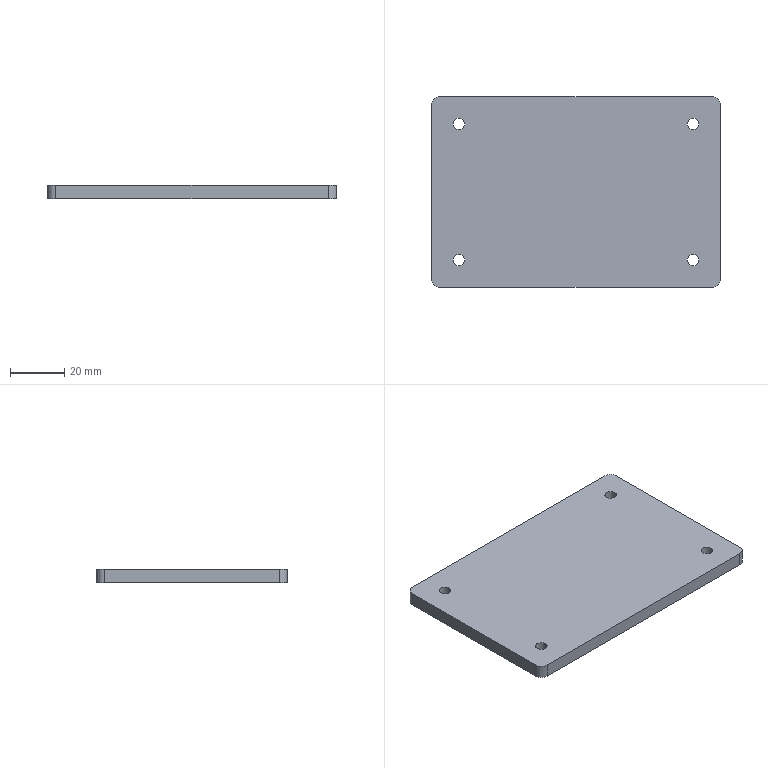Part | SolidWorks | features Extrusion 1, Fillet 1, ICE 1 | 1 solid | 18 faces | box 106 x 70 x 5 mm | volume 36784 mm3 | cylinder 12 | plane 6 | commonest cylinder face diameters 4.2 x8 6 x4
STEP:
#1=CARTESIAN_POINT('',(40.9,25.,-2.5));
#2=VERTEX_POINT('',#1);
#3=CARTESIAN_POINT('',(45.1,25.,-2.5));
#4=VERTEX_POINT('',#3);
#5=CARTESIAN_POINT('',(43.,25.,-2.5));
#6=DIRECTION('',(0.,0.,1.));
#7=DIRECTION('',(-1.,0.,0.));
#8=AXIS2_PLACEMENT_3D('',#5,#6,#7);
#9=CIRCLE('',#8,2.1);
#10=EDGE_CURVE('',#2,#4,#9,.T.);
#11=ORIENTED_EDGE('',*,*,#10,.F.);
#12=CARTESIAN_POINT('',(40.9,25.,2.5));
#13=VERTEX_POINT('',#12);
#14=CARTESIAN_POINT('',(40.9,25.,-2.5));
#15=DIRECTION('',(0.,0.,1.));
#16=VECTOR('',#15,1000.);
#17=LINE('',#14,#16);
#18=EDGE_CURVE('',#2,#13,#17,.T.);
#19=ORIENTED_EDGE('',*,*,#18,.T.);
#20=CARTESIAN_POINT('',(45.1,25.,2.5));
#21=VERTEX_POINT('',#20);
#22=CARTESIAN_POINT('',(43.,25.,2.5));
#23=DIRECTION('',(0.,0.,1.));
#24=DIRECTION('',(-1.,0.,0.));
#25=AXIS2_PLACEMENT_3D('',#22,#23,#24);
#26=CIRCLE('',#25,2.1);
#27=EDGE_CURVE('',#13,#21,#26,.T.);
#28=ORIENTED_EDGE('',*,*,#27,.T.);
#29=CARTESIAN_POINT('',(45.1,25.,-2.5));
#30=DIRECTION('',(0.,0.,1.));
#31=VECTOR('',#30,1000.);
#32=LINE('',#29,#31);
#33=EDGE_CURVE('',#4,#21,#32,.T.);
#34=ORIENTED_EDGE('',*,*,#33,.F.);
#35=EDGE_LOOP('',(#11,#19,#28,#34));
#36=FACE_OUTER_BOUND('',#35,.T.);
#37=CARTESIAN_POINT('',(43.,25.,-2.5));
#38=DIRECTION('',(0.,0.,1.));
#39=DIRECTION('',(1.,0.,0.));
#40=AXIS2_PLACEMENT_3D('',#37,#38,#39);
#41=CYLINDRICAL_SURFACE('',#40,2.1);
#42=ADVANCED_FACE('',(#36),#41,.F.);
#43=CARTESIAN_POINT('',(40.9,-25.,-2.5));
#44=VERTEX_POINT('',#43);
#45=CARTESIAN_POINT('',(45.1,-25.,-2.5));
#46=VERTEX_POINT('',#45);
#47=CARTESIAN_POINT('',(43.,-25.,-2.5));
#48=DIRECTION('',(0.,0.,1.));
#49=DIRECTION('',(1.,0.,0.));
#50=AXIS2_PLACEMENT_3D('',#47,#48,#49);
#51=CIRCLE('',#50,2.1);
#52=EDGE_CURVE('',#44,#46,#51,.T.);
#53=ORIENTED_EDGE('',*,*,#52,.F.);
#54=CARTESIAN_POINT('',(40.9,-25.,2.5));
#55=VERTEX_POINT('',#54);
#56=CARTESIAN_POINT('',(40.9,-25.,-2.5));
#57=DIRECTION('',(0.,0.,1.));
#58=VECTOR('',#57,1000.);
#59=LINE('',#56,#58);
#60=EDGE_CURVE('',#44,#55,#59,.T.);
#61=ORIENTED_EDGE('',*,*,#60,.T.);
#62=CARTESIAN_POINT('',(45.1,-25.,2.5));
#63=VERTEX_POINT('',#62);
#64=CARTESIAN_POINT('',(43.,-25.,2.5));
#65=DIRECTION('',(0.,0.,1.));
#66=DIRECTION('',(1.,0.,0.));
#67=AXIS2_PLACEMENT_3D('',#64,#65,#66);
#68=CIRCLE('',#67,2.1);
#69=EDGE_CURVE('',#55,#63,#68,.T.);
#70=ORIENTED_EDGE('',*,*,#69,.T.);
#71=CARTESIAN_POINT('',(45.1,-25.,-2.5));
#72=DIRECTION('',(0.,0.,1.));
#73=VECTOR('',#72,1000.);
#74=LINE('',#71,#73);
#75=EDGE_CURVE('',#46,#63,#74,.T.);
#76=ORIENTED_EDGE('',*,*,#75,.F.);
#77=EDGE_LOOP('',(#53,#61,#70,#76));
#78=FACE_OUTER_BOUND('',#77,.T.);
#79=CARTESIAN_POINT('',(43.,-25.,-2.5));
#80=DIRECTION('',(0.,0.,1.));
#81=DIRECTION('',(1.,0.,0.));
#82=AXIS2_PLACEMENT_3D('',#79,#80,#81);
#83=CYLINDRICAL_SURFACE('',#82,2.1);
#84=ADVANCED_FACE('',(#78),#83,.F.);
#85=CARTESIAN_POINT('',(-45.1,-25.,-2.5));
#86=VERTEX_POINT('',#85);
#87=CARTESIAN_POINT('',(-40.9,-25.,-2.5));
#88=VERTEX_POINT('',#87);
#89=CARTESIAN_POINT('',(-43.,-25.,-2.5));
#90=DIRECTION('',(0.,0.,1.));
#91=DIRECTION('',(-1.,0.,0.));
#92=AXIS2_PLACEMENT_3D('',#89,#90,#91);
#93=CIRCLE('',#92,2.1);
#94=EDGE_CURVE('',#86,#88,#93,.T.);
#95=ORIENTED_EDGE('',*,*,#94,.F.);
#96=CARTESIAN_POINT('',(-45.1,-25.,2.5));
#97=VERTEX_POINT('',#96);
#98=CARTESIAN_POINT('',(-45.1,-25.,-2.5));
#99=DIRECTION('',(0.,0.,1.));
#100=VECTOR('',#99,1000.);
#101=LINE('',#98,#100);
#102=EDGE_CURVE('',#86,#97,#101,.T.);
#103=ORIENTED_EDGE('',*,*,#102,.T.);
#104=CARTESIAN_POINT('',(-40.9,-25.,2.5));
#105=VERTEX_POINT('',#104);
#106=CARTESIAN_POINT('',(-43.,-25.,2.5));
#107=DIRECTION('',(0.,0.,1.));
#108=DIRECTION('',(-1.,0.,0.));
#109=AXIS2_PLACEMENT_3D('',#106,#107,#108);
#110=CIRCLE('',#109,2.1);
#111=EDGE_CURVE('',#97,#105,#110,.T.);
#112=ORIENTED_EDGE('',*,*,#111,.T.);
#113=CARTESIAN_POINT('',(-40.9,-25.,-2.5));
#114=DIRECTION('',(0.,0.,1.));
#115=VECTOR('',#114,1000.);
#116=LINE('',#113,#115);
#117=EDGE_CURVE('',#88,#105,#116,.T.);
#118=ORIENTED_EDGE('',*,*,#117,.F.);
#119=EDGE_LOOP('',(#95,#103,#112,#118));
#120=FACE_OUTER_BOUND('',#119,.T.);
#121=CARTESIAN_POINT('',(-43.,-25.,-2.5));
#122=DIRECTION('',(0.,0.,1.));
#123=DIRECTION('',(1.,0.,0.));
#124=AXIS2_PLACEMENT_3D('',#121,#122,#123);
#125=CYLINDRICAL_SURFACE('',#124,2.1);
#126=ADVANCED_FACE('',(#120),#125,.F.);
#127=CARTESIAN_POINT('',(-45.1,25.,-2.5));
#128=VERTEX_POINT('',#127);
#129=CARTESIAN_POINT('',(-40.9,25.,-2.5));
#130=VERTEX_POINT('',#129);
#131=CARTESIAN_POINT('',(-43.,25.,-2.5));
#132=DIRECTION('',(0.,0.,1.));
#133=DIRECTION('',(1.,0.,0.));
#134=AXIS2_PLACEMENT_3D('',#131,#132,#133);
#135=CIRCLE('',#134,2.1);
#136=EDGE_CURVE('',#128,#130,#135,.T.);
#137=ORIENTED_EDGE('',*,*,#136,.F.);
#138=CARTESIAN_POINT('',(-45.1,25.,2.5));
#139=VERTEX_POINT('',#138);
#140=CARTESIAN_POINT('',(-45.1,25.,-2.5));
#141=DIRECTION('',(0.,0.,1.));
#142=VECTOR('',#141,1000.);
#143=LINE('',#140,#142);
#144=EDGE_CURVE('',#128,#139,#143,.T.);
#145=ORIENTED_EDGE('',*,*,#144,.T.);
#146=CARTESIAN_POINT('',(-40.9,25.,2.5));
#147=VERTEX_POINT('',#146);
#148=CARTESIAN_POINT('',(-43.,25.,2.5));
#149=DIRECTION('',(0.,0.,1.));
#150=DIRECTION('',(1.,0.,0.));
#151=AXIS2_PLACEMENT_3D('',#148,#149,#150);
#152=CIRCLE('',#151,2.1);
#153=EDGE_CURVE('',#139,#147,#152,.T.);
#154=ORIENTED_EDGE('',*,*,#153,.T.);
#155=CARTESIAN_POINT('',(-40.9,25.,-2.5));
#156=DIRECTION('',(0.,0.,1.));
#157=VECTOR('',#156,1000.);
#158=LINE('',#155,#157);
#159=EDGE_CURVE('',#130,#147,#158,.T.);
#160=ORIENTED_EDGE('',*,*,#159,.F.);
#161=EDGE_LOOP('',(#137,#145,#154,#160));
#162=FACE_OUTER_BOUND('',#161,.T.);
#163=CARTESIAN_POINT('',(-43.,25.,-2.5));
#164=DIRECTION('',(0.,0.,1.));
#165=DIRECTION('',(1.,0.,0.));
#166=AXIS2_PLACEMENT_3D('',#163,#164,#165);
#167=CYLINDRICAL_SURFACE('',#166,2.1);
#168=ADVANCED_FACE('',(#162),#167,.F.);
#169=CARTESIAN_POINT('',(53.,-32.,2.5));
#170=VERTEX_POINT('',#169);
#171=CARTESIAN_POINT('',(53.,32.,2.5));
#172=VERTEX_POINT('',#171);
#173=CARTESIAN_POINT('',(53.,35.,2.5));
#174=DIRECTION('',(0.,1.,0.));
#175=VECTOR('',#174,1000.);
#176=LINE('',#173,#175);
#177=EDGE_CURVE('',#170,#172,#176,.T.);
#178=ORIENTED_EDGE('',*,*,#177,.F.);
#179=CARTESIAN_POINT('',(53.,-32.,-2.5));
#180=VERTEX_POINT('',#179);
#181=CARTESIAN_POINT('',(53.,-32.,2.5));
#182=DIRECTION('',(0.,0.,-1.));
#183=VECTOR('',#182,1000.);
#184=LINE('',#181,#183);
#185=EDGE_CURVE('',#170,#180,#184,.T.);
#186=ORIENTED_EDGE('',*,*,#185,.T.);
#187=CARTESIAN_POINT('',(53.,32.,-2.5));
#188=VERTEX_POINT('',#187);
#189=CARTESIAN_POINT('',(53.,35.,-2.5));
#190=DIRECTION('',(0.,1.,0.));
#191=VECTOR('',#190,1000.);
#192=LINE('',#189,#191);
#193=EDGE_CURVE('',#180,#188,#192,.T.);
#194=ORIENTED_EDGE('',*,*,#193,.T.);
#195=CARTESIAN_POINT('',(53.,32.,2.5));
#196=DIRECTION('',(0.,0.,1.));
#197=VECTOR('',#196,1000.);
#198=LINE('',#195,#197);
#199=EDGE_CURVE('',#188,#172,#198,.T.);
#200=ORIENTED_EDGE('',*,*,#199,.T.);
#201=EDGE_LOOP('',(#178,#186,#194,#200));
#202=FACE_OUTER_BOUND('',#201,.T.);
#203=CARTESIAN_POINT('',(53.,35.,2.5));
#204=DIRECTION('',(-1.,0.,0.));
#205=DIRECTION('',(0.,0.,1.));
#206=AXIS2_PLACEMENT_3D('',#203,#204,#205);
#207=PLANE('',#206);
#208=ADVANCED_FACE('',(#202),#207,.F.);
#209=CARTESIAN_POINT('',(50.,35.,2.5));
#210=VERTEX_POINT('',#209);
#211=CARTESIAN_POINT('',(-50.,35.,2.5));
#212=VERTEX_POINT('',#211);
#213=CARTESIAN_POINT('',(-53.,35.,2.5));
#214=DIRECTION('',(-1.,0.,0.));
#215=VECTOR('',#214,1000.);
#216=LINE('',#213,#215);
#217=EDGE_CURVE('',#210,#212,#216,.T.);
#218=ORIENTED_EDGE('',*,*,#217,.F.);
#219=CARTESIAN_POINT('',(50.,35.,-2.5));
#220=VERTEX_POINT('',#219);
#221=CARTESIAN_POINT('',(50.,35.,2.5));
#222=DIRECTION('',(0.,0.,-1.));
#223=VECTOR('',#222,1000.);
#224=LINE('',#221,#223);
#225=EDGE_CURVE('',#210,#220,#224,.T.);
#226=ORIENTED_EDGE('',*,*,#225,.T.);
#227=CARTESIAN_POINT('',(-50.,35.,-2.5));
#228=VERTEX_POINT('',#227);
#229=CARTESIAN_POINT('',(-53.,35.,-2.5));
#230=DIRECTION('',(-1.,0.,0.));
#231=VECTOR('',#230,1000.);
#232=LINE('',#229,#231);
#233=EDGE_CURVE('',#220,#228,#232,.T.);
#234=ORIENTED_EDGE('',*,*,#233,.T.);
#235=CARTESIAN_POINT('',(-50.,35.,2.5));
#236=DIRECTION('',(0.,0.,1.));
#237=VECTOR('',#236,1000.);
#238=LINE('',#235,#237);
#239=EDGE_CURVE('',#228,#212,#238,.T.);
#240=ORIENTED_EDGE('',*,*,#239,.T.);
#241=EDGE_LOOP('',(#218,#226,#234,#240));
#242=FACE_OUTER_BOUND('',#241,.T.);
#243=CARTESIAN_POINT('',(-53.,35.,2.5));
#244=DIRECTION('',(0.,-1.,0.));
#245=DIRECTION('',(0.,0.,-1.));
#246=AXIS2_PLACEMENT_3D('',#243,#244,#245);
#247=PLANE('',#246);
#248=ADVANCED_FACE('',(#242),#247,.F.);
#249=CARTESIAN_POINT('',(-53.,32.,-2.5));
#250=VERTEX_POINT('',#249);
#251=CARTESIAN_POINT('',(-53.,-32.,-2.5));
#252=VERTEX_POINT('',#251);
#253=CARTESIAN_POINT('',(-53.,35.,-2.5));
#254=DIRECTION('',(0.,-1.,0.));
#255=VECTOR('',#254,1000.);
#256=LINE('',#253,#255);
#257=EDGE_CURVE('',#250,#252,#256,.T.);
#258=ORIENTED_EDGE('',*,*,#257,.T.);
#259=CARTESIAN_POINT('',(-53.,-32.,2.5));
#260=VERTEX_POINT('',#259);
#261=CARTESIAN_POINT('',(-53.,-32.,2.5));
#262=DIRECTION('',(0.,0.,1.));
#263=VECTOR('',#262,1000.);
#264=LINE('',#261,#263);
#265=EDGE_CURVE('',#252,#260,#264,.T.);
#266=ORIENTED_EDGE('',*,*,#265,.T.);
#267=CARTESIAN_POINT('',(-53.,32.,2.5));
#268=VERTEX_POINT('',#267);
#269=CARTESIAN_POINT('',(-53.,35.,2.5));
#270=DIRECTION('',(0.,-1.,0.));
#271=VECTOR('',#270,1000.);
#272=LINE('',#269,#271);
#273=EDGE_CURVE('',#268,#260,#272,.T.);
#274=ORIENTED_EDGE('',*,*,#273,.F.);
#275=CARTESIAN_POINT('',(-53.,32.,2.5));
#276=DIRECTION('',(0.,0.,-1.));
#277=VECTOR('',#276,1000.);
#278=LINE('',#275,#277);
#279=EDGE_CURVE('',#268,#250,#278,.T.);
#280=ORIENTED_EDGE('',*,*,#279,.T.);
#281=EDGE_LOOP('',(#258,#266,#274,#280));
#282=FACE_OUTER_BOUND('',#281,.T.);
#283=CARTESIAN_POINT('',(-53.,35.,2.5));
#284=DIRECTION('',(1.,0.,0.));
#285=DIRECTION('',(0.,0.,-1.));
#286=AXIS2_PLACEMENT_3D('',#283,#284,#285);
#287=PLANE('',#286);
#288=ADVANCED_FACE('',(#282),#287,.F.);
#289=CARTESIAN_POINT('',(-50.,-35.,2.5));
#290=VERTEX_POINT('',#289);
#291=CARTESIAN_POINT('',(50.,-35.,2.5));
#292=VERTEX_POINT('',#291);
#293=CARTESIAN_POINT('',(-53.,-35.,2.5));
#294=DIRECTION('',(1.,0.,0.));
#295=VECTOR('',#294,1000.);
#296=LINE('',#293,#295);
#297=EDGE_CURVE('',#290,#292,#296,.T.);
#298=ORIENTED_EDGE('',*,*,#297,.F.);
#299=CARTESIAN_POINT('',(-50.,-35.,-2.5));
#300=VERTEX_POINT('',#299);
#301=CARTESIAN_POINT('',(-50.,-35.,2.5));
#302=DIRECTION('',(0.,0.,-1.));
#303=VECTOR('',#302,1000.);
#304=LINE('',#301,#303);
#305=EDGE_CURVE('',#290,#300,#304,.T.);
#306=ORIENTED_EDGE('',*,*,#305,.T.);
#307=CARTESIAN_POINT('',(50.,-35.,-2.5));
#308=VERTEX_POINT('',#307);
#309=CARTESIAN_POINT('',(-53.,-35.,-2.5));
#310=DIRECTION('',(1.,0.,0.));
#311=VECTOR('',#310,1000.);
#312=LINE('',#309,#311);
#313=EDGE_CURVE('',#300,#308,#312,.T.);
#314=ORIENTED_EDGE('',*,*,#313,.T.);
#315=CARTESIAN_POINT('',(50.,-35.,2.5));
#316=DIRECTION('',(0.,0.,1.));
#317=VECTOR('',#316,1000.);
#318=LINE('',#315,#317);
#319=EDGE_CURVE('',#308,#292,#318,.T.);
#320=ORIENTED_EDGE('',*,*,#319,.T.);
#321=EDGE_LOOP('',(#298,#306,#314,#320));
#322=FACE_OUTER_BOUND('',#321,.T.);
#323=CARTESIAN_POINT('',(-53.,-35.,2.5));
#324=DIRECTION('',(0.,1.,0.));
#325=DIRECTION('',(0.,0.,1.));
#326=AXIS2_PLACEMENT_3D('',#323,#324,#325);
#327=PLANE('',#326);
#328=ADVANCED_FACE('',(#322),#327,.F.);
#329=CARTESIAN_POINT('',(43.,25.,2.5));
#330=DIRECTION('',(0.,0.,1.));
#331=DIRECTION('',(-1.,0.,0.));
#332=AXIS2_PLACEMENT_3D('',#329,#330,#331);
#333=CIRCLE('',#332,2.1);
#334=EDGE_CURVE('',#21,#13,#333,.T.);
#335=ORIENTED_EDGE('',*,*,#334,.F.);
#336=ORIENTED_EDGE('',*,*,#27,.F.);
#337=EDGE_LOOP('',(#335,#336));
#338=FACE_BOUND('',#337,.T.);
#339=CARTESIAN_POINT('',(43.,-25.,2.5));
#340=DIRECTION('',(0.,0.,1.));
#341=DIRECTION('',(1.,0.,0.));
#342=AXIS2_PLACEMENT_3D('',#339,#340,#341);
#343=CIRCLE('',#342,2.1);
#344=EDGE_CURVE('',#63,#55,#343,.T.);
#345=ORIENTED_EDGE('',*,*,#344,.F.);
#346=ORIENTED_EDGE('',*,*,#69,.F.);
#347=EDGE_LOOP('',(#345,#346));
#348=FACE_BOUND('',#347,.T.);
#349=CARTESIAN_POINT('',(-43.,-25.,2.5));
#350=DIRECTION('',(0.,0.,1.));
#351=DIRECTION('',(-1.,0.,0.));
#352=AXIS2_PLACEMENT_3D('',#349,#350,#351);
#353=CIRCLE('',#352,2.1);
#354=EDGE_CURVE('',#105,#97,#353,.T.);
#355=ORIENTED_EDGE('',*,*,#354,.F.);
#356=ORIENTED_EDGE('',*,*,#111,.F.);
#357=EDGE_LOOP('',(#355,#356));
#358=FACE_BOUND('',#357,.T.);
#359=CARTESIAN_POINT('',(-43.,25.,2.5));
#360=DIRECTION('',(0.,0.,1.));
#361=DIRECTION('',(1.,0.,0.));
#362=AXIS2_PLACEMENT_3D('',#359,#360,#361);
#363=CIRCLE('',#362,2.1);
#364=EDGE_CURVE('',#147,#139,#363,.T.);
#365=ORIENTED_EDGE('',*,*,#364,.F.);
#366=ORIENTED_EDGE('',*,*,#153,.F.);
#367=EDGE_LOOP('',(#365,#366));
#368=FACE_BOUND('',#367,.T.);
#369=ORIENTED_EDGE('',*,*,#273,.T.);
#370=CARTESIAN_POINT('',(-50.,-32.,2.5));
#371=DIRECTION('',(0.,0.,1.));
#372=DIRECTION('',(1.,0.,0.));
#373=AXIS2_PLACEMENT_3D('',#370,#371,#372);
#374=CIRCLE('',#373,3.);
#375=EDGE_CURVE('',#260,#290,#374,.T.);
#376=ORIENTED_EDGE('',*,*,#375,.T.);
#377=ORIENTED_EDGE('',*,*,#297,.T.);
#378=CARTESIAN_POINT('',(50.,-32.,2.5));
#379=DIRECTION('',(0.,0.,1.));
#380=DIRECTION('',(1.,0.,0.));
#381=AXIS2_PLACEMENT_3D('',#378,#379,#380);
#382=CIRCLE('',#381,3.);
#383=EDGE_CURVE('',#292,#170,#382,.T.);
#384=ORIENTED_EDGE('',*,*,#383,.T.);
#385=ORIENTED_EDGE('',*,*,#177,.T.);
#386=CARTESIAN_POINT('',(50.,32.,2.5));
#387=DIRECTION('',(0.,0.,1.));
#388=DIRECTION('',(1.,0.,0.));
#389=AXIS2_PLACEMENT_3D('',#386,#387,#388);
#390=CIRCLE('',#389,3.);
#391=EDGE_CURVE('',#172,#210,#390,.T.);
#392=ORIENTED_EDGE('',*,*,#391,.T.);
#393=ORIENTED_EDGE('',*,*,#217,.T.);
#394=CARTESIAN_POINT('',(-50.,32.,2.5));
#395=DIRECTION('',(0.,0.,1.));
#396=DIRECTION('',(1.,0.,0.));
#397=AXIS2_PLACEMENT_3D('',#394,#395,#396);
#398=CIRCLE('',#397,3.);
#399=EDGE_CURVE('',#212,#268,#398,.T.);
#400=ORIENTED_EDGE('',*,*,#399,.T.);
#401=EDGE_LOOP('',(#369,#376,#377,#384,#385,#392,#393,#400));
#402=FACE_OUTER_BOUND('',#401,.T.);
#403=CARTESIAN_POINT('',(0.,0.,2.5));
#404=DIRECTION('',(0.,0.,1.));
#405=DIRECTION('',(1.,0.,0.));
#406=AXIS2_PLACEMENT_3D('',#403,#404,#405);
#407=PLANE('',#406);
#408=ADVANCED_FACE('',(#338,#348,#358,#368,#402),#407,.T.);
#409=CARTESIAN_POINT('',(43.,25.,-2.5));
#410=DIRECTION('',(0.,0.,1.));
#411=DIRECTION('',(-1.,0.,0.));
#412=AXIS2_PLACEMENT_3D('',#409,#410,#411);
#413=CIRCLE('',#412,2.1);
#414=EDGE_CURVE('',#4,#2,#413,.T.);
#415=ORIENTED_EDGE('',*,*,#414,.T.);
#416=ORIENTED_EDGE('',*,*,#10,.T.);
#417=EDGE_LOOP('',(#415,#416));
#418=FACE_BOUND('',#417,.T.);
#419=CARTESIAN_POINT('',(43.,-25.,-2.5));
#420=DIRECTION('',(0.,0.,1.));
#421=DIRECTION('',(1.,0.,0.));
#422=AXIS2_PLACEMENT_3D('',#419,#420,#421);
#423=CIRCLE('',#422,2.1);
#424=EDGE_CURVE('',#46,#44,#423,.T.);
#425=ORIENTED_EDGE('',*,*,#424,.T.);
#426=ORIENTED_EDGE('',*,*,#52,.T.);
#427=EDGE_LOOP('',(#425,#426));
#428=FACE_BOUND('',#427,.T.);
#429=CARTESIAN_POINT('',(-43.,-25.,-2.5));
#430=DIRECTION('',(0.,0.,1.));
#431=DIRECTION('',(-1.,0.,0.));
#432=AXIS2_PLACEMENT_3D('',#429,#430,#431);
#433=CIRCLE('',#432,2.1);
#434=EDGE_CURVE('',#88,#86,#433,.T.);
#435=ORIENTED_EDGE('',*,*,#434,.T.);
#436=ORIENTED_EDGE('',*,*,#94,.T.);
#437=EDGE_LOOP('',(#435,#436));
#438=FACE_BOUND('',#437,.T.);
#439=CARTESIAN_POINT('',(-43.,25.,-2.5));
#440=DIRECTION('',(0.,0.,1.));
#441=DIRECTION('',(1.,0.,0.));
#442=AXIS2_PLACEMENT_3D('',#439,#440,#441);
#443=CIRCLE('',#442,2.1);
#444=EDGE_CURVE('',#130,#128,#443,.T.);
#445=ORIENTED_EDGE('',*,*,#444,.T.);
#446=ORIENTED_EDGE('',*,*,#136,.T.);
#447=EDGE_LOOP('',(#445,#446));
#448=FACE_BOUND('',#447,.T.);
#449=ORIENTED_EDGE('',*,*,#313,.F.);
#450=CARTESIAN_POINT('',(-50.,-32.,-2.5));
#451=DIRECTION('',(0.,0.,-1.));
#452=DIRECTION('',(1.,0.,0.));
#453=AXIS2_PLACEMENT_3D('',#450,#451,#452);
#454=CIRCLE('',#453,3.);
#455=EDGE_CURVE('',#300,#252,#454,.T.);
#456=ORIENTED_EDGE('',*,*,#455,.T.);
#457=ORIENTED_EDGE('',*,*,#257,.F.);
#458=CARTESIAN_POINT('',(-50.,32.,-2.5));
#459=DIRECTION('',(0.,0.,-1.));
#460=DIRECTION('',(1.,0.,0.));
#461=AXIS2_PLACEMENT_3D('',#458,#459,#460);
#462=CIRCLE('',#461,3.);
#463=EDGE_CURVE('',#250,#228,#462,.T.);
#464=ORIENTED_EDGE('',*,*,#463,.T.);
#465=ORIENTED_EDGE('',*,*,#233,.F.);
#466=CARTESIAN_POINT('',(50.,32.,-2.5));
#467=DIRECTION('',(0.,0.,-1.));
#468=DIRECTION('',(1.,0.,0.));
#469=AXIS2_PLACEMENT_3D('',#466,#467,#468);
#470=CIRCLE('',#469,3.);
#471=EDGE_CURVE('',#220,#188,#470,.T.);
#472=ORIENTED_EDGE('',*,*,#471,.T.);
#473=ORIENTED_EDGE('',*,*,#193,.F.);
#474=CARTESIAN_POINT('',(50.,-32.,-2.5));
#475=DIRECTION('',(0.,0.,-1.));
#476=DIRECTION('',(1.,0.,0.));
#477=AXIS2_PLACEMENT_3D('',#474,#475,#476);
#478=CIRCLE('',#477,3.);
#479=EDGE_CURVE('',#180,#308,#478,.T.);
#480=ORIENTED_EDGE('',*,*,#479,.T.);
#481=EDGE_LOOP('',(#449,#456,#457,#464,#465,#472,#473,#480));
#482=FACE_OUTER_BOUND('',#481,.T.);
#483=CARTESIAN_POINT('',(0.,0.,-2.5));
#484=DIRECTION('',(0.,0.,1.));
#485=DIRECTION('',(1.,0.,0.));
#486=AXIS2_PLACEMENT_3D('',#483,#484,#485);
#487=PLANE('',#486);
#488=ADVANCED_FACE('',(#418,#428,#438,#448,#482),#487,.F.);
#489=ORIENTED_EDGE('',*,*,#144,.F.);
#490=ORIENTED_EDGE('',*,*,#444,.F.);
#491=ORIENTED_EDGE('',*,*,#159,.T.);
#492=ORIENTED_EDGE('',*,*,#364,.T.);
#493=EDGE_LOOP('',(#489,#490,#491,#492));
#494=FACE_OUTER_BOUND('',#493,.T.);
#495=CARTESIAN_POINT('',(-43.,25.,-2.5));
#496=DIRECTION('',(0.,0.,1.));
#497=DIRECTION('',(1.,0.,0.));
#498=AXIS2_PLACEMENT_3D('',#495,#496,#497);
#499=CYLINDRICAL_SURFACE('',#498,2.1);
#500=ADVANCED_FACE('',(#494),#499,.F.);
#501=ORIENTED_EDGE('',*,*,#102,.F.);
#502=ORIENTED_EDGE('',*,*,#434,.F.);
#503=ORIENTED_EDGE('',*,*,#117,.T.);
#504=ORIENTED_EDGE('',*,*,#354,.T.);
#505=EDGE_LOOP('',(#501,#502,#503,#504));
#506=FACE_OUTER_BOUND('',#505,.T.);
#507=CARTESIAN_POINT('',(-43.,-25.,-2.5));
#508=DIRECTION('',(0.,0.,1.));
#509=DIRECTION('',(1.,0.,0.));
#510=AXIS2_PLACEMENT_3D('',#507,#508,#509);
#511=CYLINDRICAL_SURFACE('',#510,2.1);
#512=ADVANCED_FACE('',(#506),#511,.F.);
#513=ORIENTED_EDGE('',*,*,#60,.F.);
#514=ORIENTED_EDGE('',*,*,#424,.F.);
#515=ORIENTED_EDGE('',*,*,#75,.T.);
#516=ORIENTED_EDGE('',*,*,#344,.T.);
#517=EDGE_LOOP('',(#513,#514,#515,#516));
#518=FACE_OUTER_BOUND('',#517,.T.);
#519=CARTESIAN_POINT('',(43.,-25.,-2.5));
#520=DIRECTION('',(0.,0.,1.));
#521=DIRECTION('',(1.,0.,0.));
#522=AXIS2_PLACEMENT_3D('',#519,#520,#521);
#523=CYLINDRICAL_SURFACE('',#522,2.1);
#524=ADVANCED_FACE('',(#518),#523,.F.);
#525=ORIENTED_EDGE('',*,*,#18,.F.);
#526=ORIENTED_EDGE('',*,*,#414,.F.);
#527=ORIENTED_EDGE('',*,*,#33,.T.);
#528=ORIENTED_EDGE('',*,*,#334,.T.);
#529=EDGE_LOOP('',(#525,#526,#527,#528));
#530=FACE_OUTER_BOUND('',#529,.T.);
#531=CARTESIAN_POINT('',(43.,25.,-2.5));
#532=DIRECTION('',(0.,0.,1.));
#533=DIRECTION('',(1.,0.,0.));
#534=AXIS2_PLACEMENT_3D('',#531,#532,#533);
#535=CYLINDRICAL_SURFACE('',#534,2.1);
#536=ADVANCED_FACE('',(#530),#535,.F.);
#537=ORIENTED_EDGE('',*,*,#375,.F.);
#538=ORIENTED_EDGE('',*,*,#265,.F.);
#539=ORIENTED_EDGE('',*,*,#455,.F.);
#540=ORIENTED_EDGE('',*,*,#305,.F.);
#541=EDGE_LOOP('',(#537,#538,#539,#540));
#542=FACE_OUTER_BOUND('',#541,.T.);
#543=CARTESIAN_POINT('',(-50.,-32.,2.5));
#544=DIRECTION('',(0.,0.,-1.));
#545=DIRECTION('',(-1.,0.,0.));
#546=AXIS2_PLACEMENT_3D('',#543,#544,#545);
#547=CYLINDRICAL_SURFACE('',#546,3.);
#548=ADVANCED_FACE('',(#542),#547,.T.);
#549=ORIENTED_EDGE('',*,*,#383,.F.);
#550=ORIENTED_EDGE('',*,*,#319,.F.);
#551=ORIENTED_EDGE('',*,*,#479,.F.);
#552=ORIENTED_EDGE('',*,*,#185,.F.);
#553=EDGE_LOOP('',(#549,#550,#551,#552));
#554=FACE_OUTER_BOUND('',#553,.T.);
#555=CARTESIAN_POINT('',(50.,-32.,2.5));
#556=DIRECTION('',(0.,0.,-1.));
#557=DIRECTION('',(-1.,0.,0.));
#558=AXIS2_PLACEMENT_3D('',#555,#556,#557);
#559=CYLINDRICAL_SURFACE('',#558,3.);
#560=ADVANCED_FACE('',(#554),#559,.T.);
#561=ORIENTED_EDGE('',*,*,#391,.F.);
#562=ORIENTED_EDGE('',*,*,#199,.F.);
#563=ORIENTED_EDGE('',*,*,#471,.F.);
#564=ORIENTED_EDGE('',*,*,#225,.F.);
#565=EDGE_LOOP('',(#561,#562,#563,#564));
#566=FACE_OUTER_BOUND('',#565,.T.);
#567=CARTESIAN_POINT('',(50.,32.,2.5));
#568=DIRECTION('',(0.,0.,-1.));
#569=DIRECTION('',(-1.,0.,0.));
#570=AXIS2_PLACEMENT_3D('',#567,#568,#569);
#571=CYLINDRICAL_SURFACE('',#570,3.);
#572=ADVANCED_FACE('',(#566),#571,.T.);
#573=ORIENTED_EDGE('',*,*,#399,.F.);
#574=ORIENTED_EDGE('',*,*,#239,.F.);
#575=ORIENTED_EDGE('',*,*,#463,.F.);
#576=ORIENTED_EDGE('',*,*,#279,.F.);
#577=EDGE_LOOP('',(#573,#574,#575,#576));
#578=FACE_OUTER_BOUND('',#577,.T.);
#579=CARTESIAN_POINT('',(-50.,32.,2.5));
#580=DIRECTION('',(0.,0.,-1.));
#581=DIRECTION('',(-1.,0.,0.));
#582=AXIS2_PLACEMENT_3D('',#579,#580,#581);
#583=CYLINDRICAL_SURFACE('',#582,3.);
#584=ADVANCED_FACE('',(#578),#583,.T.);
#585=CLOSED_SHELL('',(#42,#84,#126,#168,#208,#248,#288,#328,#408,#488,#500,#512,#524,#536,#548,#560,#572,#584));
#586=MANIFOLD_SOLID_BREP('',#585);
#587=CARTESIAN_POINT('',(0.,0.,0.));
#588=DIRECTION('',(0.,0.,1.));
#589=DIRECTION('',(1.,0.,0.));
#590=AXIS2_PLACEMENT_3D('',#587,#588,#589);
#591=(LENGTH_UNIT()NAMED_UNIT(*)SI_UNIT(.MILLI.,.METRE.));
#592=UNCERTAINTY_MEASURE_WITH_UNIT(LENGTH_MEASURE(0.00001),#591,'','');
#593=(NAMED_UNIT(*)PLANE_ANGLE_UNIT()SI_UNIT($,.RADIAN.));
#594=(NAMED_UNIT(*)SI_UNIT($,.STERADIAN.)SOLID_ANGLE_UNIT());
#595=(GEOMETRIC_REPRESENTATION_CONTEXT(3)GLOBAL_UNCERTAINTY_ASSIGNED_CONTEXT((#592))GLOBAL_UNIT_ASSIGNED_CONTEXT((#591,#593,#594))REPRESENTATION_CONTEXT('',''));
#596=ADVANCED_BREP_SHAPE_REPRESENTATION('',(#586,#590),#595);